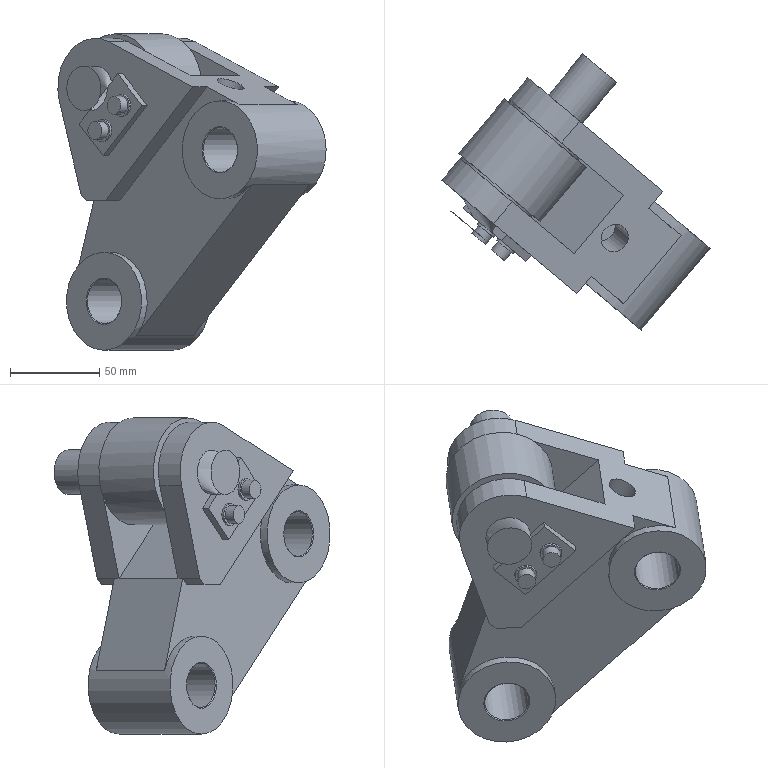Part | NX | features solid 2 | 2 solids | 62 faces | box 150.522 x 154.943 x 177.5 mm | volume 860193 mm3 | plane 37 | cylinder 17 | cone 8 | commonest cylinder face diameters 25 x5 55 x4 10 x2 12.2 x2 48 x2 16 x1